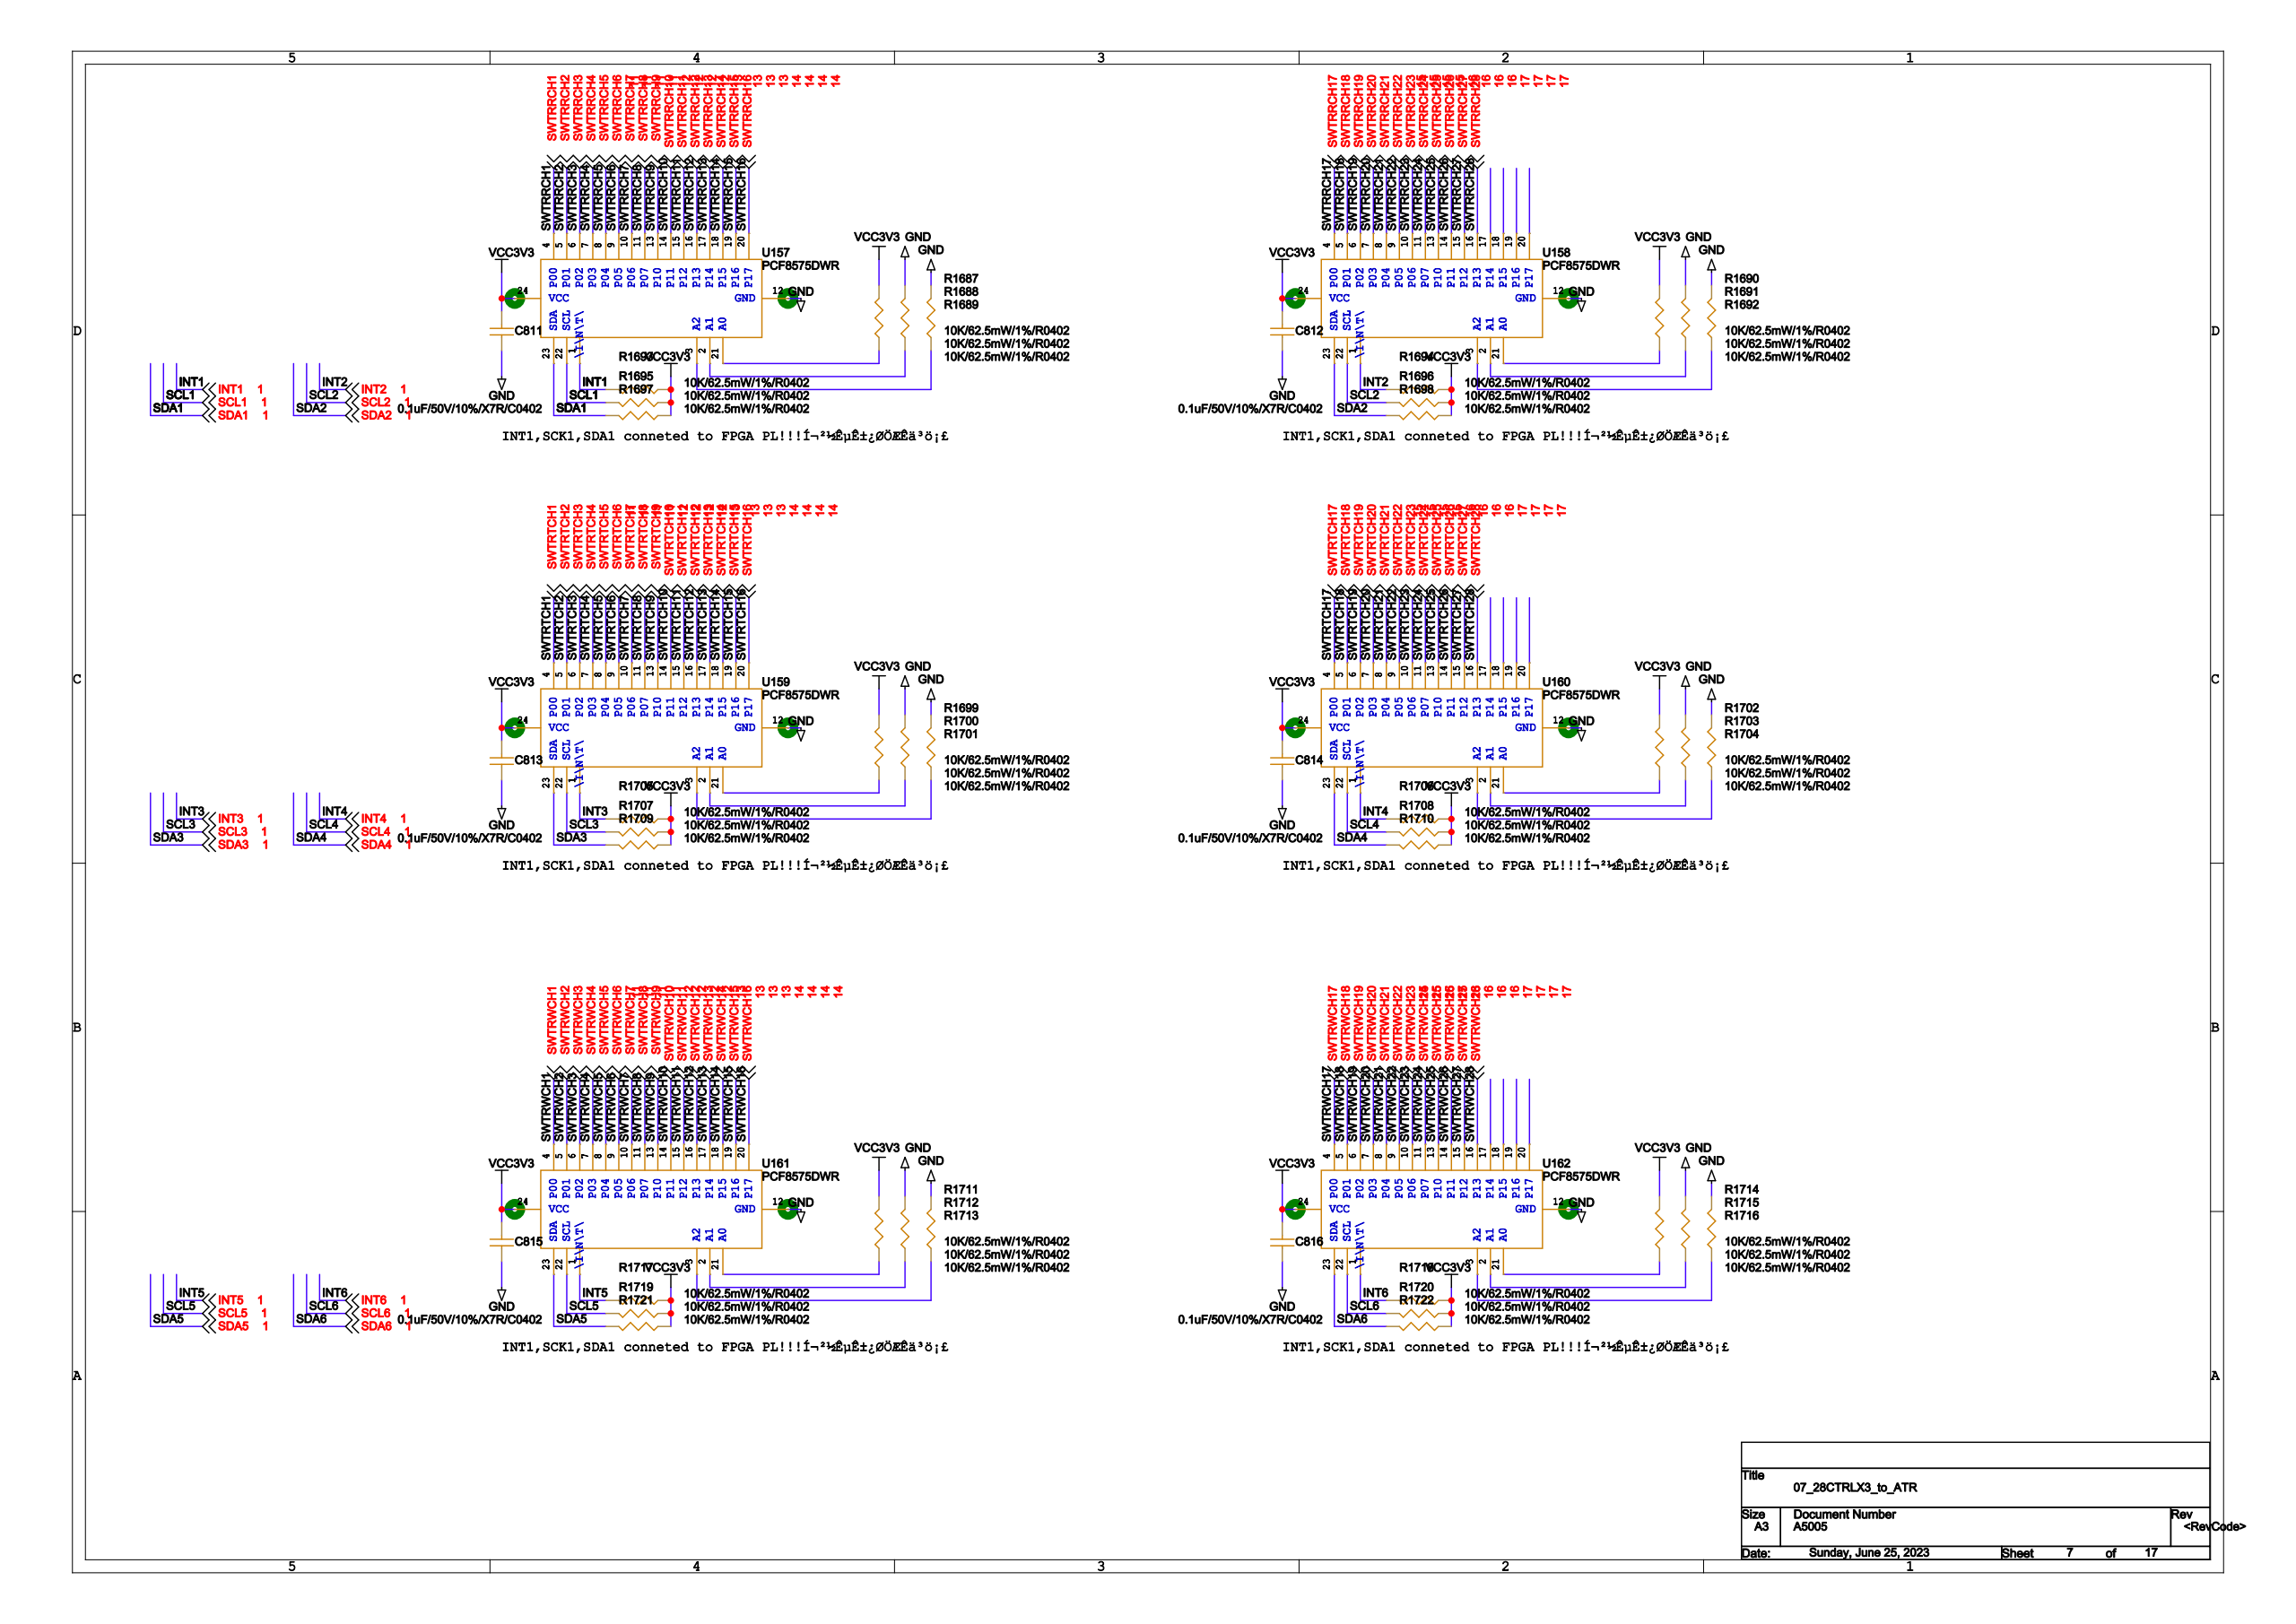Circuit board | Cadence Allegro | 2002 parts | 1538 nets | one sheet of the schematic
Parts on this sheet (reference | value | footprint):
C811 | 0.1uF/50V/10%/X7R/C0402 | 0402
C812 | 0.1uF/50V/10%/X7R/C0402 | 0402
C813 | 0.1uF/50V/10%/X7R/C0402 | 0402
C814 | 0.1uF/50V/10%/X7R/C0402 | 0402
C815 | 0.1uF/50V/10%/X7R/C0402 | 0402
C816 | 0.1uF/50V/10%/X7R/C0402 | 0402
R1687 | 10K/62.5mW/1%/R0402 | 0402
R1688 | 10K/62.5mW/1%/R0402 | 0402
R1689 | 10K/62.5mW/1%/R0402 | 0402
R1690 | 10K/62.5mW/1%/R0402 | 0402
R1691 | 10K/62.5mW/1%/R0402 | 0402
R1692 | 10K/62.5mW/1%/R0402 | 0402
R1693 | 10K/62.5mW/1%/R0402 | 0402
R1694 | 10K/62.5mW/1%/R0402 | 0402
R1695 | 10K/62.5mW/1%/R0402 | 0402
R1696 | 10K/62.5mW/1%/R0402 | 0402
R1697 | 10K/62.5mW/1%/R0402 | 0402
R1698 | 10K/62.5mW/1%/R0402 | 0402
R1699 | 10K/62.5mW/1%/R0402 | 0402
R1700 | 10K/62.5mW/1%/R0402 | 0402
R1701 | 10K/62.5mW/1%/R0402 | 0402
R1702 | 10K/62.5mW/1%/R0402 | 0402
R1703 | 10K/62.5mW/1%/R0402 | 0402
R1704 | 10K/62.5mW/1%/R0402 | 0402
R1705 | 10K/62.5mW/1%/R0402 | 0402
R1706 | 10K/62.5mW/1%/R0402 | 0402
R1707 | 10K/62.5mW/1%/R0402 | 0402
R1708 | 10K/62.5mW/1%/R0402 | 0402
R1709 | 10K/62.5mW/1%/R0402 | 0402
R1710 | 10K/62.5mW/1%/R0402 | 0402
R1711 | 10K/62.5mW/1%/R0402 | 0402
R1712 | 10K/62.5mW/1%/R0402 | 0402
R1713 | 10K/62.5mW/1%/R0402 | 0402
R1714 | 10K/62.5mW/1%/R0402 | 0402
R1715 | 10K/62.5mW/1%/R0402 | 0402
R1716 | 10K/62.5mW/1%/R0402 | 0402
R1717 | 10K/62.5mW/1%/R0402 | 0402
R1718 | 10K/62.5mW/1%/R0402 | 0402
R1719 | 10K/62.5mW/1%/R0402 | 0402
R1720 | 10K/62.5mW/1%/R0402 | 0402
R1721 | 10K/62.5mW/1%/R0402 | 0402
R1722 | 10K/62.5mW/1%/R0402 | 0402
U157 | PCF8575DWR | SOIC_24
U158 | PCF8575DWR | SOIC_24
U159 | PCF8575DWR | SOIC_24
U160 | PCF8575DWR | SOIC_24
U161 | PCF8575DWR | SOIC_24
U162 | PCF8575DWR | SOIC_24
Nets of these parts (net: part-pin ...):
3.3V: C811-2 C812-2 C813-2 C814-2 C815-2 C816-2 R1687-1 R1690-1 R1693-2 R1694-2 R1695-2 R1696-2 R1697-2 R1698-2 R1699-1 R1702-1 R1705-2 R1706-2 R1707-2 R1708-2 R1709-2 R1710-2 R1711-1 R1714-1 R1717-2 R1718-2 R1719-2 R1720-2 R1721-2 R1722-2 U157-24 U158-24 U159-24 U160-24 U161-24 U162-24
AGND: C811-1 C812-1 C813-1 C814-1 C815-1 C816-1 R1688-1 R1689-1 R1691-1 R1692-1 R1700-1 R1701-1 R1703-1 R1704-1 R1712-1 R1713-1 R1715-1 R1716-1 U157-12 U158-12 U159-12 U160-12 U161-12 U162-12
SCL6: R1720-1 U162-22
INT6: R1718-1 U162-1
INT5: R1717-1 U161-1
SDA5: R1721-1 U161-23
SCL5: R1719-1 U161-22
SDA4: R1710-1 U160-23
SCL4: R1708-1 U160-22
INT4: R1706-1 U160-1
SDA3: R1709-1 U159-23
SCL3: R1707-1 U159-22
INT3: R1705-1 U159-1
INT1: R1693-1 U157-1
SDA1: R1697-1 U157-23
SCL1: R1695-1 U157-22
SDA6: R1722-1 U162-23
SDA2: R1698-1 U158-23
SCL2: R1696-1 U158-22
INT2: R1694-1 U158-1
SWTRTCH1: U159-4
SWTRRCH1: U157-4
SWTRWCH1: U161-4
SWTRWCH2: U161-5
SWTRRCH2: U157-5
SWTRTCH2: U159-5
SWTRRCH3: U157-6
SWTRTCH3: U159-6
SWTRWCH3: U161-6
SWTRRCH4: U157-7
SWTRTCH4: U159-7
SWTRWCH4: U161-7
SWTRTCH5: U159-8
SWTRWCH5: U161-8
SWTRRCH5: U157-8
SWTRRCH6: U157-9
SWTRTCH6: U159-9
SWTRWCH6: U161-9
SWTRRCH7: U157-10
SWTRTCH7: U159-10
SWTRWCH7: U161-10
SWTRRCH8: U157-11
SWTRTCH8: U159-11
SWTRWCH8: U161-11
SWTRRCH9: U157-13
SWTRTCH9: U159-13
SWTRWCH9: U161-13
SWTRTCH10: U159-14
SWTRRCH10: U157-14
SWTRWCH10: U161-14
SWTRRCH11: U157-15
SWTRTCH11: U159-15
SWTRWCH11: U161-15
SWTRRCH12: U157-16
SWTRTCH12: U159-16
SWTRWCH12: U161-16
SWTRTCH13: U159-17
SWTRRCH13: U157-17
SWTRWCH13: U161-17
SWTRRCH14: U157-18
SWTRTCH14: U159-18
SWTRWCH14: U161-18
SWTRRCH15: U157-19
SWTRTCH15: U159-19
SWTRWCH15: U161-19
SWTRRCH16: U157-20
SWTRTCH16: U159-20
SWTRWCH16: U161-20
SWTRTCH17: U160-4
SWTRRCH17: U158-4
SWTRWCH17: U162-4
SWTRRCH18: U158-5
SWTRTCH18: U160-5
SWTRWCH18: U162-5
SWTRRCH19: U158-6
SWTRTCH19: U160-6
SWTRWCH19: U162-6
SWTRRCH20: U158-7
SWTRTCH20: U160-7
SWTRWCH20: U162-7
SWTRTCH21: U160-8
SWTRWCH21: U162-8
SWTRRCH21: U158-8
SWTRRCH22: U158-9
SWTRTCH22: U160-9
SWTRWCH22: U162-9
SWTRRCH23: U158-10
SWTRWCH23: U162-10
SWTRTCH23: U160-10
SWTRRCH24: U158-11
SWTRTCH24: U160-11
SWTRWCH24: U162-11
SWTRTCH25: U160-13
SWTRRCH25: U158-13
SWTRWCH25: U162-13
SWTRRCH26: U158-14
SWTRTCH26: U160-14
SWTRWCH26: U162-14
SWTRTCH27: U160-15
SWTRRCH27: U158-15
SWTRWCH27: U162-15
SWTRRCH28: U158-16
SWTRTCH28: U160-16
SWTRWCH28: U162-16
N23855480: R1687-2 U157-21
N23855482: R1688-2 U157-2
N23855484: R1689-2 U157-3
N23856166: R1690-2 U158-21
N23856168: R1691-2 U158-2
N23856170: R1692-2 U158-3
N23988542: R1699-2 U159-21
N23988544: R1700-2 U159-2
N23988546: R1701-2 U159-3
N23988042: R1702-2 U160-21
N23988044: R1703-2 U160-2
N23988046: R1704-2 U160-3
N23990137: R1711-2 U161-21
N23990139: R1712-2 U161-2
N23990141: R1713-2 U161-3
N23989637: R1714-2 U162-21
N23989639: R1715-2 U162-2
N23989641: R1716-2 U162-3